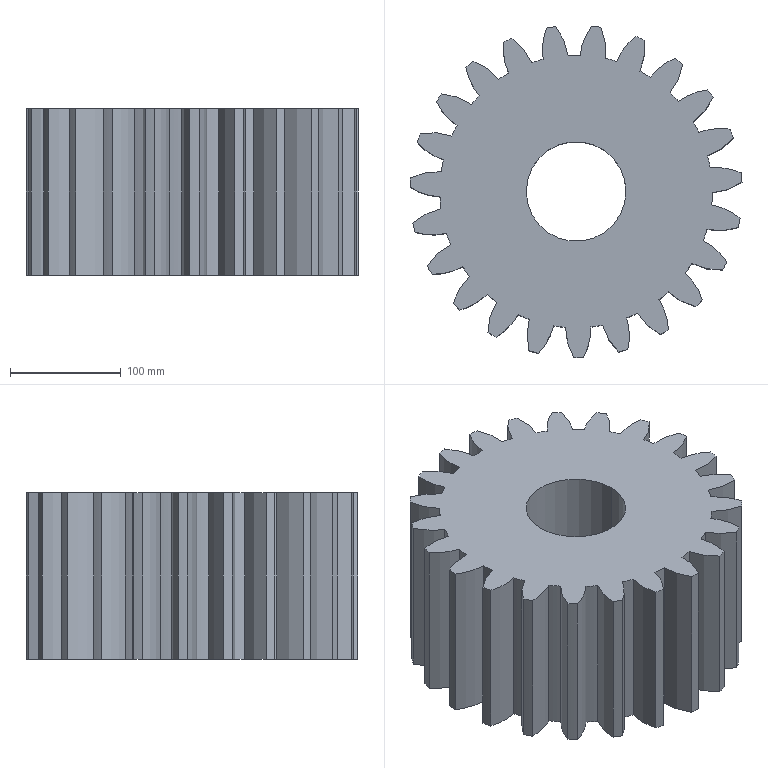Part | SolidWorks | features ICE 2, CirPattern 1, Extrusion 1 | 1 solid | 96 faces | box 299.728 x 299.348 x 150 mm | volume 7864200 mm3 | cylinder 48 | spline 46 | plane 2 | commonest cylinder face diameters 246 x23 300 x23 90 x2